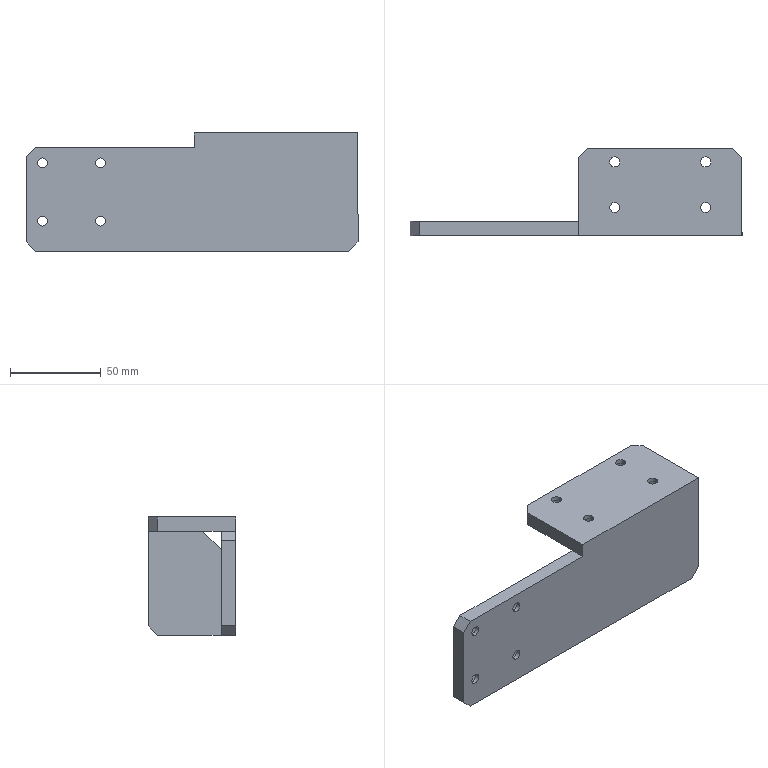Part | SolidWorks | features BaseBody 1 | 1 solid | 59 faces | box 182.664 x 48 x 65 mm | volume 131076 mm3 | cylinder 32 | plane 27 | commonest cylinder face diameters 5.5 x16 10 x16